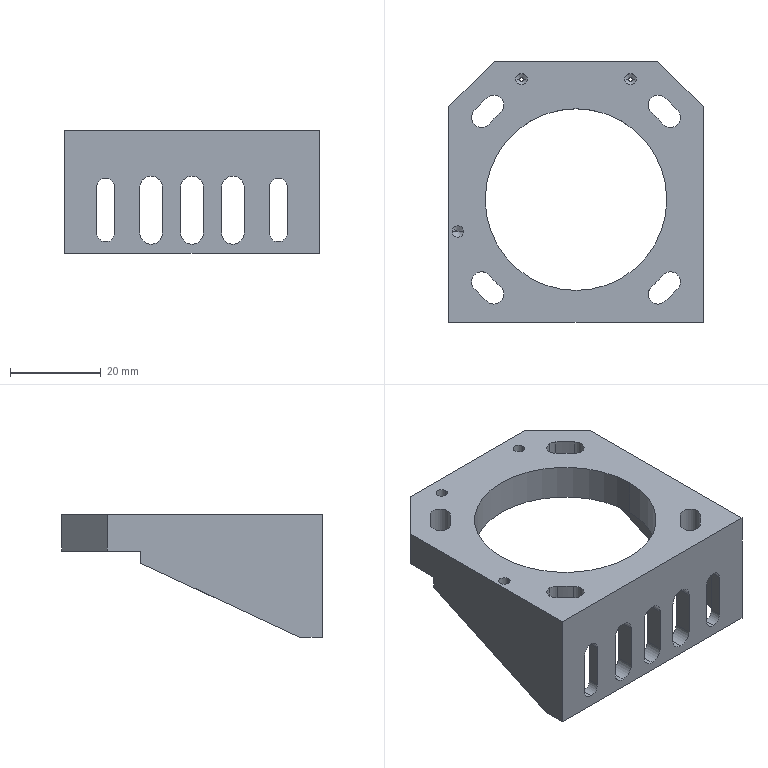NC program | NX | posted with a generic post | part box 56 x 57.4 x 27 mm
Lines 31 to 1094 of 24340:
(ZLEVEL_PROFILE , TOOL : D10C)
N54 T10 M6
N56 G54
N58 G17 G0 G90 X-33.8 Y5.489 B0. C0. S2500 M3
N60 G43 Z30. H10
N62 Z1.5
N64 G94 G1 Y28.32 Z0.303 F1000.
N66 X-33.683 Y29.131 Z0.261
N68 X-33.438 Y29.914 Z0.218
N70 X-33.071 Y30.647 Z0.175
N72 X-32.592 Y31.312 Z0.132
N74 X-32.012 Y31.892 Z0.089
N76 X-31.347 Y32.371 Z0.046
N78 X-30.614 Y32.738 Z0.003
N80 X-29.831 Y32.983 Z-0.04
N82 X-29.02 Y33.1 Z-0.083
N84 X-28.7 Z-0.1
N86 X18.7 F2500.
N88 G2 X22.306 Y31.606 R5.1
N90 G1 X32.306 Y21.606
N92 G2 X33.8 Y18. R5.1
N94 G1 Y-18.
N96 G2 X32.306 Y-21.606 R5.1
N98 G1 X22.306 Y-31.606
N100 G2 X18.7 Y-33.1 R5.1
N102 G1 X-28.7
N104 G2 X-33.8 Y-28. R5.1
N106 G1 Y28.
N108 G2 X-28.7 Y33.1 R5.1
N110 G1 X-22.971 Z-0.2
N112 X18.7
N114 G2 X22.306 Y31.606 R5.1
N116 G1 X32.306 Y21.606
N118 G2 X33.8 Y18. R5.1
N120 G1 Y-18.
N122 G2 X32.306 Y-21.606 R5.1
N124 G1 X22.306 Y-31.606
N126 G2 X18.7 Y-33.1 R5.1
N128 G1 X-28.7
N130 G2 X-33.8 Y-28. R5.1
N132 G1 Y28.
N134 G2 X-28.7 Y33.1 R5.1
N136 G1 X-22.971 Z-0.3
N138 X18.7
N140 G2 X22.306 Y31.606 R5.1
N142 G1 X32.306 Y21.606
N144 G2 X33.8 Y18. R5.1
N146 G1 Y-18.
N148 G2 X32.306 Y-21.606 R5.1
N150 G1 X22.306 Y-31.606
N152 G2 X18.7 Y-33.1 R5.1
N154 G1 X-28.7
N156 G2 X-33.8 Y-28. R5.1
N158 G1 Y28.
N160 G2 X-28.7 Y33.1 R5.1
N162 G1 X-22.971 Z-0.4
N164 X18.7
N166 G2 X22.306 Y31.606 R5.1
N168 G1 X32.306 Y21.606
N170 G2 X33.8 Y18. R5.1
N172 G1 Y-18.
N174 G2 X32.306 Y-21.606 R5.1
N176 G1 X22.306 Y-31.606
N178 G2 X18.7 Y-33.1 R5.1
N180 G1 X-28.7
N182 G2 X-33.8 Y-28. R5.1
N184 G1 Y28.
N186 G2 X-28.7 Y33.1 R5.1
N188 G1 X-22.971 Z-0.5
N190 X18.7
N192 G2 X22.306 Y31.606 R5.1
N194 G1 X32.306 Y21.606
N196 G2 X33.8 Y18. R5.1
N198 G1 Y-18.
N200 G2 X32.306 Y-21.606 R5.1
N202 G1 X22.306 Y-31.606
N204 G2 X18.7 Y-33.1 R5.1
N206 G1 X-28.7
N208 G2 X-33.8 Y-28. R5.1
N210 G1 Y28.
N212 G2 X-28.7 Y33.1 R5.1
N214 G1 X-22.971 Z-0.6
N216 X18.7
N218 G2 X22.306 Y31.606 R5.1
N220 G1 X32.306 Y21.606
N222 G2 X33.8 Y18. R5.1
N224 G1 Y-18.
N226 G2 X32.306 Y-21.606 R5.1
N228 G1 X22.306 Y-31.606
N230 G2 X18.7 Y-33.1 R5.1
N232 G1 X-28.7
N234 G2 X-33.8 Y-28. R5.1
N236 G1 Y28.
N238 G2 X-28.7 Y33.1 R5.1
N240 G1 X-22.971 Z-0.7
N242 X18.7
N244 G2 X22.306 Y31.606 R5.1
N246 G1 X32.306 Y21.606
N248 G2 X33.8 Y18. R5.1
N250 G1 Y-18.
N252 G2 X32.306 Y-21.606 R5.1
N254 G1 X22.306 Y-31.606
N256 G2 X18.7 Y-33.1 R5.1
N258 G1 X-28.7
N260 G2 X-33.8 Y-28. R5.1
N262 G1 Y28.
N264 G2 X-28.7 Y33.1 R5.1
N266 G1 X-22.971 Z-0.8
N268 X18.7
N270 G2 X22.306 Y31.606 R5.1
N272 G1 X32.306 Y21.606
N274 G2 X33.8 Y18. R5.1
N276 G1 Y-18.
N278 G2 X32.306 Y-21.606 R5.1
N280 G1 X22.306 Y-31.606
N282 G2 X18.7 Y-33.1 R5.1
N284 G1 X-28.7
N286 G2 X-33.8 Y-28. R5.1
N288 G1 Y28.
N290 G2 X-28.7 Y33.1 R5.1
N292 G1 X-22.971 Z-0.9
N294 X18.7
N296 G2 X22.306 Y31.606 R5.1
N298 G1 X32.306 Y21.606
N300 G2 X33.8 Y18. R5.1
N302 G1 Y-18.
N304 G2 X32.306 Y-21.606 R5.1
N306 G1 X22.306 Y-31.606
N308 G2 X18.7 Y-33.1 R5.1
N310 G1 X-28.7
N312 G2 X-33.8 Y-28. R5.1
N314 G1 Y28.
N316 G2 X-28.7 Y33.1 R5.1
N318 G1 X-22.971 Z-1.
N320 X18.7
N322 G2 X22.306 Y31.606 R5.1
N324 G1 X32.306 Y21.606
N326 G2 X33.8 Y18. R5.1
N328 G1 Y-18.
N330 G2 X32.306 Y-21.606 R5.1
N332 G1 X22.306 Y-31.606
N334 G2 X18.7 Y-33.1 R5.1
N336 G1 X-28.7
N338 G2 X-33.8 Y-28. R5.1
N340 G1 Y28.
N342 G2 X-28.7 Y33.1 R5.1
N344 G1 X-22.971 Z-1.1
N346 X18.7
N348 G2 X22.306 Y31.606 R5.1
N350 G1 X32.306 Y21.606
N352 G2 X33.8 Y18. R5.1
N354 G1 Y-18.
N356 G2 X32.306 Y-21.606 R5.1
N358 G1 X22.306 Y-31.606
N360 G2 X18.7 Y-33.1 R5.1
N362 G1 X-28.7
N364 G2 X-33.8 Y-28. R5.1
N366 G1 Y28.
N368 G2 X-28.7 Y33.1 R5.1
N370 G1 X-22.971 Z-1.2
N372 X18.7
N374 G2 X22.306 Y31.606 R5.1
N376 G1 X32.306 Y21.606
N378 G2 X33.8 Y18. R5.1
N380 G1 Y-18.
N382 G2 X32.306 Y-21.606 R5.1
N384 G1 X22.306 Y-31.606
N386 G2 X18.7 Y-33.1 R5.1
N388 G1 X-28.7
N390 G2 X-33.8 Y-28. R5.1
N392 G1 Y28.
N394 G2 X-28.7 Y33.1 R5.1
N396 G1 X-22.971 Z-1.3
N398 X18.7
N400 G2 X22.306 Y31.606 R5.1
N402 G1 X32.306 Y21.606
N404 G2 X33.8 Y18. R5.1
N406 G1 Y-18.
N408 G2 X32.306 Y-21.606 R5.1
N410 G1 X22.306 Y-31.606
N412 G2 X18.7 Y-33.1 R5.1
N414 G1 X-28.7
N416 G2 X-33.8 Y-28. R5.1
N418 G1 Y28.
N420 G2 X-28.7 Y33.1 R5.1
N422 G1 X-22.971 Z-1.4
N424 X18.7
N426 G2 X22.306 Y31.606 R5.1
N428 G1 X32.306 Y21.606
N430 G2 X33.8 Y18. R5.1
N432 G1 Y-18.
N434 G2 X32.306 Y-21.606 R5.1
N436 G1 X22.306 Y-31.606
N438 G2 X18.7 Y-33.1 R5.1
N440 G1 X-28.7
N442 G2 X-33.8 Y-28. R5.1
N444 G1 Y28.
N446 G2 X-28.7 Y33.1 R5.1
N448 G1 X-22.971 Z-1.5
N450 X18.7
N452 G2 X22.306 Y31.606 R5.1
N454 G1 X32.306 Y21.606
N456 G2 X33.8 Y18. R5.1
N458 G1 Y-18.
N460 G2 X32.306 Y-21.606 R5.1
N462 G1 X22.306 Y-31.606
N464 G2 X18.7 Y-33.1 R5.1
N466 G1 X-28.7
N468 G2 X-33.8 Y-28. R5.1
N470 G1 Y28.
N472 G2 X-28.7 Y33.1 R5.1
N474 G1 X-22.971 Z-1.6
N476 X18.7
N478 G2 X22.306 Y31.606 R5.1
N480 G1 X32.306 Y21.606
N482 G2 X33.8 Y18. R5.1
N484 G1 Y-18.
N486 G2 X32.306 Y-21.606 R5.1
N488 G1 X22.306 Y-31.606
N490 G2 X18.7 Y-33.1 R5.1
N492 G1 X-28.7
N494 G2 X-33.8 Y-28. R5.1
N496 G1 Y28.
N498 G2 X-28.7 Y33.1 R5.1
N500 G1 X-22.971 Z-1.7
N502 X18.7
N504 G2 X22.306 Y31.606 R5.1
N506 G1 X32.306 Y21.606
N508 G2 X33.8 Y18. R5.1
N510 G1 Y-18.
N512 G2 X32.306 Y-21.606 R5.1
N514 G1 X22.306 Y-31.606
N516 G2 X18.7 Y-33.1 R5.1
N518 G1 X-28.7
N520 G2 X-33.8 Y-28. R5.1
N522 G1 Y28.
N524 G2 X-28.7 Y33.1 R5.1
N526 G1 X-22.971 Z-1.8
N528 X18.7
N530 G2 X22.306 Y31.606 R5.1
N532 G1 X32.306 Y21.606
N534 G2 X33.8 Y18. R5.1
N536 G1 Y-18.
N538 G2 X32.306 Y-21.606 R5.1
N540 G1 X22.306 Y-31.606
N542 G2 X18.7 Y-33.1 R5.1
N544 G1 X-28.7
N546 G2 X-33.8 Y-28. R5.1
N548 G1 Y28.
N550 G2 X-28.7 Y33.1 R5.1
N552 G1 X-22.971 Z-1.9
N554 X18.7
N556 G2 X22.306 Y31.606 R5.1
N558 G1 X32.306 Y21.606
N560 G2 X33.8 Y18. R5.1
N562 G1 Y-18.
N564 G2 X32.306 Y-21.606 R5.1
N566 G1 X22.306 Y-31.606
N568 G2 X18.7 Y-33.1 R5.1
N570 G1 X-28.7
N572 G2 X-33.8 Y-28. R5.1
N574 G1 Y28.
N576 G2 X-28.7 Y33.1 R5.1
N578 G1 X-22.971 Z-2.
N580 X18.7
N582 G2 X22.306 Y31.606 R5.1
N584 G1 X32.306 Y21.606
N586 G2 X33.8 Y18. R5.1
N588 G1 Y-18.
N590 G2 X32.306 Y-21.606 R5.1
N592 G1 X22.306 Y-31.606
N594 G2 X18.7 Y-33.1 R5.1
N596 G1 X-28.7
N598 G2 X-33.8 Y-28. R5.1
N600 G1 Y28.
N602 G2 X-28.7 Y33.1 R5.1
N604 G1 X-22.971 Z-2.1
N606 X18.7
N608 G2 X22.306 Y31.606 R5.1
N610 G1 X32.306 Y21.606
N612 G2 X33.8 Y18. R5.1
N614 G1 Y-18.
N616 G2 X32.306 Y-21.606 R5.1
N618 G1 X22.306 Y-31.606
N620 G2 X18.7 Y-33.1 R5.1
N622 G1 X-28.7
N624 G2 X-33.8 Y-28. R5.1
N626 G1 Y28.
N628 G2 X-28.7 Y33.1 R5.1
N630 G1 X-22.971 Z-2.2
N632 X18.7
N634 G2 X22.306 Y31.606 R5.1
N636 G1 X32.306 Y21.606
N638 G2 X33.8 Y18. R5.1
N640 G1 Y-18.
N642 G2 X32.306 Y-21.606 R5.1
N644 G1 X22.306 Y-31.606
N646 G2 X18.7 Y-33.1 R5.1
N648 G1 X-28.7
N650 G2 X-33.8 Y-28. R5.1
N652 G1 Y28.
N654 G2 X-28.7 Y33.1 R5.1
N656 G1 X-22.971 Z-2.3
N658 X18.7
N660 G2 X22.306 Y31.606 R5.1
N662 G1 X32.306 Y21.606
N664 G2 X33.8 Y18. R5.1
N666 G1 Y-18.
N668 G2 X32.306 Y-21.606 R5.1
N670 G1 X22.306 Y-31.606
N672 G2 X18.7 Y-33.1 R5.1
N674 G1 X-28.7
N676 G2 X-33.8 Y-28. R5.1
N678 G1 Y28.
N680 G2 X-28.7 Y33.1 R5.1
N682 G1 X-22.971 Z-2.4
N684 X18.7
N686 G2 X22.306 Y31.606 R5.1
N688 G1 X32.306 Y21.606
N690 G2 X33.8 Y18. R5.1
N692 G1 Y-18.
N694 G2 X32.306 Y-21.606 R5.1
N696 G1 X22.306 Y-31.606
N698 G2 X18.7 Y-33.1 R5.1
N700 G1 X-28.7
N702 G2 X-33.8 Y-28. R5.1
N704 G1 Y28.
N706 G2 X-28.7 Y33.1 R5.1
N708 G1 X-22.971 Z-2.5
N710 X18.7
N712 G2 X22.306 Y31.606 R5.1
N714 G1 X32.306 Y21.606
N716 G2 X33.8 Y18. R5.1
N718 G1 Y-18.
N720 G2 X32.306 Y-21.606 R5.1
N722 G1 X22.306 Y-31.606
N724 G2 X18.7 Y-33.1 R5.1
N726 G1 X-28.7
N728 G2 X-33.8 Y-28. R5.1
N730 G1 Y28.
N732 G2 X-28.7 Y33.1 R5.1
N734 G1 X-22.971 Z-2.6
N736 X18.7
N738 G2 X22.306 Y31.606 R5.1
N740 G1 X32.306 Y21.606
N742 G2 X33.8 Y18. R5.1
N744 G1 Y-18.
N746 G2 X32.306 Y-21.606 R5.1
N748 G1 X22.306 Y-31.606
N750 G2 X18.7 Y-33.1 R5.1
N752 G1 X-28.7
N754 G2 X-33.8 Y-28. R5.1
N756 G1 Y28.
N758 G2 X-28.7 Y33.1 R5.1
N760 G1 X-22.971 Z-2.7
N762 X18.7
N764 G2 X22.306 Y31.606 R5.1
N766 G1 X32.306 Y21.606
N768 G2 X33.8 Y18. R5.1
N770 G1 Y-18.
N772 G2 X32.306 Y-21.606 R5.1
N774 G1 X22.306 Y-31.606
N776 G2 X18.7 Y-33.1 R5.1
N778 G1 X-28.7
N780 G2 X-33.8 Y-28. R5.1
N782 G1 Y28.
N784 G2 X-28.7 Y33.1 R5.1
N786 G1 X-22.971 Z-2.8
N788 X18.7
N790 G2 X22.306 Y31.606 R5.1
N792 G1 X32.306 Y21.606
N794 G2 X33.8 Y18. R5.1
N796 G1 Y-18.
N798 G2 X32.306 Y-21.606 R5.1
N800 G1 X22.306 Y-31.606
N802 G2 X18.7 Y-33.1 R5.1
N804 G1 X-28.7
N806 G2 X-33.8 Y-28. R5.1
N808 G1 Y28.
N810 G2 X-28.7 Y33.1 R5.1
N812 G1 X-22.971 Z-2.9
N814 X18.7
N816 G2 X22.306 Y31.606 R5.1
N818 G1 X32.306 Y21.606
N820 G2 X33.8 Y18. R5.1
N822 G1 Y-18.
N824 G2 X32.306 Y-21.606 R5.1
N826 G1 X22.306 Y-31.606
N828 G2 X18.7 Y-33.1 R5.1
N830 G1 X-28.7
N832 G2 X-33.8 Y-28. R5.1
N834 G1 Y28.
N836 G2 X-28.7 Y33.1 R5.1
N838 G1 X-22.971 Z-3.
N840 X18.7
N842 G2 X22.306 Y31.606 R5.1
N844 G1 X32.306 Y21.606
N846 G2 X33.8 Y18. R5.1
N848 G1 Y-18.
N850 G2 X32.306 Y-21.606 R5.1
N852 G1 X22.306 Y-31.606
N854 G2 X18.7 Y-33.1 R5.1
N856 G1 X-28.7
N858 G2 X-33.8 Y-28. R5.1
N860 G1 Y28.
N862 G2 X-28.7 Y33.1 R5.1
N864 G1 X-22.971 Z-3.1
N866 X18.7
N868 G2 X22.306 Y31.606 R5.1
N870 G1 X32.306 Y21.606
N872 G2 X33.8 Y18. R5.1
N874 G1 Y-18.
N876 G2 X32.306 Y-21.606 R5.1
N878 G1 X22.306 Y-31.606
N880 G2 X18.7 Y-33.1 R5.1
N882 G1 X-28.7
N884 G2 X-33.8 Y-28. R5.1
N886 G1 Y28.
N888 G2 X-28.7 Y33.1 R5.1
N890 G1 X-22.971 Z-3.2
N892 X18.7
N894 G2 X22.306 Y31.606 R5.1
N896 G1 X32.306 Y21.606
N898 G2 X33.8 Y18. R5.1
N900 G1 Y-18.
N902 G2 X32.306 Y-21.606 R5.1
N904 G1 X22.306 Y-31.606
N906 G2 X18.7 Y-33.1 R5.1
N908 G1 X-28.7
N910 G2 X-33.8 Y-28. R5.1
N912 G1 Y28.
N914 G2 X-28.7 Y33.1 R5.1
N916 G1 X-22.971 Z-3.3
N918 X18.7
N920 G2 X22.306 Y31.606 R5.1
N922 G1 X32.306 Y21.606
N924 G2 X33.8 Y18. R5.1
N926 G1 Y-18.
N928 G2 X32.306 Y-21.606 R5.1
N930 G1 X22.306 Y-31.606
N932 G2 X18.7 Y-33.1 R5.1
N934 G1 X-28.7
N936 G2 X-33.8 Y-28. R5.1
N938 G1 Y28.
N940 G2 X-28.7 Y33.1 R5.1
N942 G1 X-22.971 Z-3.4
N944 X18.7
N946 G2 X22.306 Y31.606 R5.1
N948 G1 X32.306 Y21.606
N950 G2 X33.8 Y18. R5.1
N952 G1 Y-18.
N954 G2 X32.306 Y-21.606 R5.1
N956 G1 X22.306 Y-31.606
N958 G2 X18.7 Y-33.1 R5.1
N960 G1 X-28.7
N962 G2 X-33.8 Y-28. R5.1
N964 G1 Y28.
N966 G2 X-28.7 Y33.1 R5.1
N968 G1 X-22.971 Z-3.5
N970 X18.7
N972 G2 X22.306 Y31.606 R5.1
N974 G1 X32.306 Y21.606
N976 G2 X33.8 Y18. R5.1
N978 G1 Y-18.
N980 G2 X32.306 Y-21.606 R5.1
N982 G1 X22.306 Y-31.606
N984 G2 X18.7 Y-33.1 R5.1
N986 G1 X-28.7
N988 G2 X-33.8 Y-28. R5.1
N990 G1 Y28.
N992 G2 X-28.7 Y33.1 R5.1
N994 G1 X-22.971 Z-3.6
N996 X18.7
N998 G2 X22.306 Y31.606 R5.1
N1000 G1 X32.306 Y21.606
N1002 G2 X33.8 Y18. R5.1
N1004 G1 Y-18.
N1006 G2 X32.306 Y-21.606 R5.1
N1008 G1 X22.306 Y-31.606
N1010 G2 X18.7 Y-33.1 R5.1
N1012 G1 X-28.7
N1014 G2 X-33.8 Y-28. R5.1
N1016 G1 Y28.
N1018 G2 X-28.7 Y33.1 R5.1
N1020 G1 X-22.971 Z-3.7
N1022 X18.7
N1024 G2 X22.306 Y31.606 R5.1
N1026 G1 X32.306 Y21.606
N1028 G2 X33.8 Y18. R5.1
N1030 G1 Y-18.
N1032 G2 X32.306 Y-21.606 R5.1
N1034 G1 X22.306 Y-31.606
N1036 G2 X18.7 Y-33.1 R5.1
N1038 G1 X-28.7
N1040 G2 X-33.8 Y-28. R5.1
N1042 G1 Y28.
N1044 G2 X-28.7 Y33.1 R5.1
N1046 G1 X-22.971 Z-3.8
N1048 X18.7
N1050 G2 X22.306 Y31.606 R5.1
N1052 G1 X32.306 Y21.606
N1054 G2 X33.8 Y18. R5.1
N1056 G1 Y-18.
N1058 G2 X32.306 Y-21.606 R5.1
N1060 G1 X22.306 Y-31.606
N1062 G2 X18.7 Y-33.1 R5.1
N1064 G1 X-28.7
N1066 G2 X-33.8 Y-28. R5.1
N1068 G1 Y28.
N1070 G2 X-28.7 Y33.1 R5.1
N1072 G1 X-22.971 Z-3.9
N1074 X18.7
N1076 G2 X22.306 Y31.606 R5.1
N1078 G1 X32.306 Y21.606
N1080 G2 X33.8 Y18. R5.1
N1082 G1 Y-18.
N1084 G2 X32.306 Y-21.606 R5.1
N1086 G1 X22.306 Y-31.606
N1088 G2 X18.7 Y-33.1 R5.1
N1090 G1 X-28.7
N1092 G2 X-33.8 Y-28. R5.1
N1094 G1 Y28.
N1096 G2 X-28.7 Y33.1 R5.1
N1098 G1 X-22.971 Z-4.
N1100 X18.7
N1102 G2 X22.306 Y31.606 R5.1
N1104 G1 X32.306 Y21.606
N1106 G2 X33.8 Y18. R5.1
N1108 G1 Y-18.
N1110 G2 X32.306 Y-21.606 R5.1
N1112 G1 X22.306 Y-31.606
N1114 G2 X18.7 Y-33.1 R5.1
N1116 G1 X-28.7
N1118 G2 X-33.8 Y-28. R5.1
N1120 G1 Y28.
N1122 G2 X-28.7 Y33.1 R5.1
N1124 G1 X-22.971 Z-4.1
N1126 X18.7
N1128 G2 X22.306 Y31.606 R5.1
N1130 G1 X32.306 Y21.606
N1132 G2 X33.8 Y18. R5.1
N1134 G1 Y-18.
N1136 G2 X32.306 Y-21.606 R5.1
N1138 G1 X22.306 Y-31.606
N1140 G2 X18.7 Y-33.1 R5.1
N1142 G1 X-28.7
N1144 G2 X-33.8 Y-28. R5.1
N1146 G1 Y28.
N1148 G2 X-28.7 Y33.1 R5.1
N1150 G1 X-22.971 Z-4.2
N1152 X18.7
N1154 G2 X22.306 Y31.606 R5.1
N1156 G1 X32.306 Y21.606
N1158 G2 X33.8 Y18. R5.1
N1160 G1 Y-18.
N1162 G2 X32.306 Y-21.606 R5.1
N1164 G1 X22.306 Y-31.606
N1166 G2 X18.7 Y-33.1 R5.1
N1168 G1 X-28.7
N1170 G2 X-33.8 Y-28. R5.1
N1172 G1 Y28.
N1174 G2 X-28.7 Y33.1 R5.1
N1176 G1 X-22.971 Z-4.3
N1178 X18.7
N1180 G2 X22.306 Y31.606 R5.1
N1182 G1 X32.306 Y21.606
N1184 G2 X33.8 Y18. R5.1
N1186 G1 Y-18.
N1188 G2 X32.306 Y-21.606 R5.1
N1190 G1 X22.306 Y-31.606
N1192 G2 X18.7 Y-33.1 R5.1
N1194 G1 X-28.7
N1196 G2 X-33.8 Y-28. R5.1
N1198 G1 Y28.
N1200 G2 X-28.7 Y33.1 R5.1
N1202 G1 X-22.971 Z-4.4
N1204 X18.7
N1206 G2 X22.306 Y31.606 R5.1
N1208 G1 X32.306 Y21.606
N1210 G2 X33.8 Y18. R5.1
N1212 G1 Y-18.
N1214 G2 X32.306 Y-21.606 R5.1
N1216 G1 X22.306 Y-31.606
N1218 G2 X18.7 Y-33.1 R5.1
N1220 G1 X-28.7
N1222 G2 X-33.8 Y-28. R5.1
N1224 G1 Y28.
N1226 G2 X-28.7 Y33.1 R5.1
N1228 G1 X-22.971 Z-4.5
N1230 X18.7
N1232 G2 X22.306 Y31.606 R5.1
N1234 G1 X32.306 Y21.606
N1236 G2 X33.8 Y18. R5.1
N1238 G1 Y-18.
N1240 G2 X32.306 Y-21.606 R5.1
N1242 G1 X22.306 Y-31.606
N1244 G2 X18.7 Y-33.1 R5.1
N1246 G1 X-28.7
N1248 G2 X-33.8 Y-28. R5.1
N1250 G1 Y28.
N1252 G2 X-28.7 Y33.1 R5.1
N1254 G1 X-22.971 Z-4.6
N1256 X18.7
N1258 G2 X22.306 Y31.606 R5.1
N1260 G1 X32.306 Y21.606
N1262 G2 X33.8 Y18. R5.1
N1264 G1 Y-18.
N1266 G2 X32.306 Y-21.606 R5.1
N1268 G1 X22.306 Y-31.606
N1270 G2 X18.7 Y-33.1 R5.1
N1272 G1 X-28.7
N1274 G2 X-33.8 Y-28. R5.1
N1276 G1 Y28.
N1278 G2 X-28.7 Y33.1 R5.1
N1280 G1 X-22.971 Z-4.7
N1282 X18.7
N1284 G2 X22.306 Y31.606 R5.1
N1286 G1 X32.306 Y21.606
N1288 G2 X33.8 Y18. R5.1
N1290 G1 Y-18.
N1292 G2 X32.306 Y-21.606 R5.1
N1294 G1 X22.306 Y-31.606
N1296 G2 X18.7 Y-33.1 R5.1
N1298 G1 X-28.7
N1300 G2 X-33.8 Y-28. R5.1
N1302 G1 Y28.
N1304 G2 X-28.7 Y33.1 R5.1
N1306 G1 X-22.971 Z-4.8
N1308 X18.7
N1310 G2 X22.306 Y31.606 R5.1
N1312 G1 X32.306 Y21.606
N1314 G2 X33.8 Y18. R5.1
N1316 G1 Y-18.
N1318 G2 X32.306 Y-21.606 R5.1
N1320 G1 X22.306 Y-31.606
N1322 G2 X18.7 Y-33.1 R5.1
N1324 G1 X-28.7
N1326 G2 X-33.8 Y-28. R5.1
N1328 G1 Y28.
N1330 G2 X-28.7 Y33.1 R5.1
N1332 G1 X-22.971 Z-4.9
N1334 X18.7
N1336 G2 X22.306 Y31.606 R5.1
N1338 G1 X32.306 Y21.606
N1340 G2 X33.8 Y18. R5.1
N1342 G1 Y-18.
N1344 G2 X32.306 Y-21.606 R5.1
N1346 G1 X22.306 Y-31.606
N1348 G2 X18.7 Y-33.1 R5.1
N1350 G1 X-28.7
N1352 G2 X-33.8 Y-28. R5.1
N1354 G1 Y28.
N1356 G2 X-28.7 Y33.1 R5.1
N1358 G1 X-22.971 Z-5.
N1360 X18.7
N1362 G2 X22.306 Y31.606 R5.1
N1364 G1 X32.306 Y21.606
N1366 G2 X33.8 Y18. R5.1
N1368 G1 Y-18.
N1370 G2 X32.306 Y-21.606 R5.1
N1372 G1 X22.306 Y-31.606
N1374 G2 X18.7 Y-33.1 R5.1
N1376 G1 X-28.7
N1378 G2 X-33.8 Y-28. R5.1
N1380 G1 Y28.
N1382 G2 X-28.7 Y33.1 R5.1
N1384 G1 X-22.971 Z-5.1
N1386 X18.7
N1388 G2 X22.306 Y31.606 R5.1
N1390 G1 X32.306 Y21.606
N1392 G2 X33.8 Y18. R5.1
N1394 G1 Y-18.
N1396 G2 X32.306 Y-21.606 R5.1
N1398 G1 X22.306 Y-31.606
N1400 G2 X18.7 Y-33.1 R5.1
N1402 G1 X-28.7
N1404 G2 X-33.8 Y-28. R5.1
N1406 G1 Y28.
N1408 G2 X-28.7 Y33.1 R5.1
N1410 G1 X-22.971 Z-5.2
N1412 X18.7
N1414 G2 X22.306 Y31.606 R5.1
N1416 G1 X32.306 Y21.606
N1418 G2 X33.8 Y18. R5.1
N1420 G1 Y-18.
N1422 G2 X32.306 Y-21.606 R5.1
N1424 G1 X22.306 Y-31.606
N1426 G2 X18.7 Y-33.1 R5.1
N1428 G1 X-28.7
N1430 G2 X-33.8 Y-28. R5.1
N1432 G1 Y28.
N1434 G2 X-28.7 Y33.1 R5.1
N1436 G1 X-22.971 Z-5.3
N1438 X18.7
N1440 G2 X22.306 Y31.606 R5.1
N1442 G1 X32.306 Y21.606
N1444 G2 X33.8 Y18. R5.1
N1446 G1 Y-18.
N1448 G2 X32.306 Y-21.606 R5.1
N1450 G1 X22.306 Y-31.606
N1452 G2 X18.7 Y-33.1 R5.1
N1454 G1 X-28.7
N1456 G2 X-33.8 Y-28. R5.1
N1458 G1 Y28.
N1460 G2 X-28.7 Y33.1 R5.1
N1462 G1 X-22.971 Z-5.4
N1464 X18.7
N1466 G2 X22.306 Y31.606 R5.1
N1468 G1 X32.306 Y21.606
N1470 G2 X33.8 Y18. R5.1
N1472 G1 Y-18.
N1474 G2 X32.306 Y-21.606 R5.1
N1476 G1 X22.306 Y-31.606
N1478 G2 X18.7 Y-33.1 R5.1
N1480 G1 X-28.7
N1482 G2 X-33.8 Y-28. R5.1
N1484 G1 Y28.
N1486 G2 X-28.7 Y33.1 R5.1
N1488 G1 X-22.971 Z-5.5
N1490 X18.7
N1492 G2 X22.306 Y31.606 R5.1
N1494 G1 X32.306 Y21.606
N1496 G2 X33.8 Y18. R5.1
N1498 G1 Y-18.
N1500 G2 X32.306 Y-21.606 R5.1
N1502 G1 X22.306 Y-31.606
N1504 G2 X18.7 Y-33.1 R5.1
N1506 G1 X-28.7
N1508 G2 X-33.8 Y-28. R5.1
N1510 G1 Y28.
N1512 G2 X-28.7 Y33.1 R5.1
N1514 G1 X-22.971 Z-5.6
N1516 X18.7
N1518 G2 X22.306 Y31.606 R5.1
N1520 G1 X32.306 Y21.606
N1522 G2 X33.8 Y18. R5.1
N1524 G1 Y-18.
N1526 G2 X32.306 Y-21.606 R5.1
N1528 G1 X22.306 Y-31.606
N1530 G2 X18.7 Y-33.1 R5.1
N1532 G1 X-28.7
N1534 G2 X-33.8 Y-28. R5.1
N1536 G1 Y28.
N1538 G2 X-28.7 Y33.1 R5.1
N1540 G1 X-22.971 Z-5.7
N1542 X18.7
N1544 G2 X22.306 Y31.606 R5.1
N1546 G1 X32.306 Y21.606
N1548 G2 X33.8 Y18. R5.1
N1550 G1 Y-18.
N1552 G2 X32.306 Y-21.606 R5.1
N1554 G1 X22.306 Y-31.606
N1556 G2 X18.7 Y-33.1 R5.1
N1558 G1 X-28.7
N1560 G2 X-33.8 Y-28. R5.1
N1562 G1 Y28.
N1564 G2 X-28.7 Y33.1 R5.1
N1566 G1 X-22.971 Z-5.8
N1568 X18.7
N1570 G2 X22.306 Y31.606 R5.1
N1572 G1 X32.306 Y21.606
N1574 G2 X33.8 Y18. R5.1
N1576 G1 Y-18.
N1578 G2 X32.306 Y-21.606 R5.1
N1580 G1 X22.306 Y-31.606
N1582 G2 X18.7 Y-33.1 R5.1
N1584 G1 X-28.7
N1586 G2 X-33.8 Y-28. R5.1
N1588 G1 Y28.
N1590 G2 X-28.7 Y33.1 R5.1
N1592 G1 X-22.971 Z-5.9
N1594 X18.7
N1596 G2 X22.306 Y31.606 R5.1
N1598 G1 X32.306 Y21.606
N1600 G2 X33.8 Y18. R5.1
N1602 G1 Y-18.
N1604 G2 X32.306 Y-21.606 R5.1
N1606 G1 X22.306 Y-31.606
N1608 G2 X18.7 Y-33.1 R5.1
N1610 G1 X-28.7
N1612 G2 X-33.8 Y-28. R5.1
N1614 G1 Y28.
N1616 G2 X-28.7 Y33.1 R5.1
N1618 G1 X-22.971 Z-6.
N1620 X18.7
N1622 G2 X22.306 Y31.606 R5.1
N1624 G1 X32.306 Y21.606
N1626 G2 X33.8 Y18. R5.1
N1628 G1 Y-18.
N1630 G2 X32.306 Y-21.606 R5.1
N1632 G1 X22.306 Y-31.606
N1634 G2 X18.7 Y-33.1 R5.1
N1636 G1 X-28.7
N1638 G2 X-33.8 Y-28. R5.1
N1640 G1 Y28.
N1642 G2 X-28.7 Y33.1 R5.1
N1644 G1 X-22.971 Z-6.1
N1646 X18.7
N1648 G2 X22.306 Y31.606 R5.1
N1650 G1 X32.306 Y21.606
N1652 G2 X33.8 Y18. R5.1
N1654 G1 Y-18.
N1656 G2 X32.306 Y-21.606 R5.1
N1658 G1 X22.306 Y-31.606
N1660 G2 X18.7 Y-33.1 R5.1
N1662 G1 X-28.7
N1664 G2 X-33.8 Y-28. R5.1
N1666 G1 Y28.
N1668 G2 X-28.7 Y33.1 R5.1
N1670 G1 X-22.971 Z-6.2
N1672 X18.7
N1674 G2 X22.306 Y31.606 R5.1
N1676 G1 X32.306 Y21.606
N1678 G2 X33.8 Y18. R5.1
N1680 G1 Y-18.
N1682 G2 X32.306 Y-21.606 R5.1
N1684 G1 X22.306 Y-31.606
N1686 G2 X18.7 Y-33.1 R5.1
N1688 G1 X-28.7
N1690 G2 X-33.8 Y-28. R5.1
N1692 G1 Y28.
N1694 G2 X-28.7 Y33.1 R5.1
N1696 G1 X-22.971 Z-6.3
N1698 X18.7
N1700 G2 X22.306 Y31.606 R5.1
N1702 G1 X32.306 Y21.606
N1704 G2 X33.8 Y18. R5.1
N1706 G1 Y-18.
N1708 G2 X32.306 Y-21.606 R5.1
N1710 G1 X22.306 Y-31.606
N1712 G2 X18.7 Y-33.1 R5.1
N1714 G1 X-28.7
N1716 G2 X-33.8 Y-28. R5.1
N1718 G1 Y28.
N1720 G2 X-28.7 Y33.1 R5.1
N1722 G1 X-22.971 Z-6.4
N1724 X18.7
N1726 G2 X22.306 Y31.606 R5.1
N1728 G1 X32.306 Y21.606
N1730 G2 X33.8 Y18. R5.1
N1732 G1 Y-18.
N1734 G2 X32.306 Y-21.606 R5.1
N1736 G1 X22.306 Y-31.606
N1738 G2 X18.7 Y-33.1 R5.1
N1740 G1 X-28.7
N1742 G2 X-33.8 Y-28. R5.1
N1744 G1 Y28.
N1746 G2 X-28.7 Y33.1 R5.1
N1748 G1 X-22.971 Z-6.5
N1750 X18.7
N1752 G2 X22.306 Y31.606 R5.1
N1754 G1 X32.306 Y21.606
N1756 G2 X33.8 Y18. R5.1
N1758 G1 Y-18.
N1760 G2 X32.306 Y-21.606 R5.1
N1762 G1 X22.306 Y-31.606
N1764 G2 X18.7 Y-33.1 R5.1
N1766 G1 X-28.7
N1768 G2 X-33.8 Y-28. R5.1
N1770 G1 Y28.
N1772 G2 X-28.7 Y33.1 R5.1
N1774 G1 X-22.971 Z-6.6
N1776 X18.7
N1778 G2 X22.306 Y31.606 R5.1
N1780 G1 X32.306 Y21.606
N1782 G2 X33.8 Y18. R5.1
N1784 G1 Y-18.
N1786 G2 X32.306 Y-21.606 R5.1
N1788 G1 X22.306 Y-31.606
N1790 G2 X18.7 Y-33.1 R5.1
N1792 G1 X-28.7
N1794 G2 X-33.8 Y-28. R5.1
N1796 G1 Y28.
N1798 G2 X-28.7 Y33.1 R5.1
N1800 G1 X-22.971 Z-6.7
N1802 X18.7
N1804 G2 X22.306 Y31.606 R5.1
N1806 G1 X32.306 Y21.606
N1808 G2 X33.8 Y18. R5.1
N1810 G1 Y-18.
N1812 G2 X32.306 Y-21.606 R5.1
N1814 G1 X22.306 Y-31.606
N1816 G2 X18.7 Y-33.1 R5.1
N1818 G1 X-28.7
N1820 G2 X-33.8 Y-28. R5.1
N1822 G1 Y28.
N1824 G2 X-28.7 Y33.1 R5.1
N1826 G1 X-22.971 Z-6.8
N1828 X18.7
N1830 G2 X22.306 Y31.606 R5.1
N1832 G1 X32.306 Y21.606
N1834 G2 X33.8 Y18. R5.1
N1836 G1 Y-18.
N1838 G2 X32.306 Y-21.606 R5.1
N1840 G1 X22.306 Y-31.606
N1842 G2 X18.7 Y-33.1 R5.1
N1844 G1 X-28.7
N1846 G2 X-33.8 Y-28. R5.1
N1848 G1 Y28.
N1850 G2 X-28.7 Y33.1 R5.1
N1852 G1 X-22.971 Z-6.9
N1854 X18.7
N1856 G2 X22.306 Y31.606 R5.1
N1858 G1 X32.306 Y21.606
N1860 G2 X33.8 Y18. R5.1
N1862 G1 Y-18.
N1864 G2 X32.306 Y-21.606 R5.1
N1866 G1 X22.306 Y-31.606
N1868 G2 X18.7 Y-33.1 R5.1
N1870 G1 X-28.7
N1872 G2 X-33.8 Y-28. R5.1
N1874 G1 Y28.
N1876 G2 X-28.7 Y33.1 R5.1
N1878 G1 X-22.971 Z-7.
N1880 X18.7
N1882 G2 X22.306 Y31.606 R5.1
N1884 G1 X32.306 Y21.606
N1886 G2 X33.8 Y18. R5.1
N1888 G1 Y-18.
N1890 G2 X32.306 Y-21.606 R5.1
N1892 G1 X22.306 Y-31.606
N1894 G2 X18.7 Y-33.1 R5.1
N1896 G1 X-28.7
N1898 G2 X-33.8 Y-28. R5.1
N1900 G1 Y28.
N1902 G2 X-28.7 Y33.1 R5.1
N1904 G1 X-22.971 Z-7.1
N1906 X18.7
N1908 G2 X22.306 Y31.606 R5.1
N1910 G1 X32.306 Y21.606
N1912 G2 X33.8 Y18. R5.1
N1914 G1 Y-18.
N1916 G2 X32.306 Y-21.606 R5.1
N1918 G1 X22.306 Y-31.606
N1920 G2 X18.7 Y-33.1 R5.1
N1922 G1 X-28.7
N1924 G2 X-33.8 Y-28. R5.1
N1926 G1 Y28.
N1928 G2 X-28.7 Y33.1 R5.1
N1930 G1 X-22.971 Z-7.2
N1932 X18.7
N1934 G2 X22.306 Y31.606 R5.1
N1936 G1 X32.306 Y21.606
N1938 G2 X33.8 Y18. R5.1
N1940 G1 Y-18.
N1942 G2 X32.306 Y-21.606 R5.1
N1944 G1 X22.306 Y-31.606
N1946 G2 X18.7 Y-33.1 R5.1
N1948 G1 X-28.7
N1950 G2 X-33.8 Y-28. R5.1
N1952 G1 Y28.
N1954 G2 X-28.7 Y33.1 R5.1
N1956 G1 X-22.971 Z-7.3
N1958 X18.7
N1960 G2 X22.306 Y31.606 R5.1
N1962 G1 X32.306 Y21.606
N1964 G2 X33.8 Y18. R5.1
N1966 G1 Y-18.
N1968 G2 X32.306 Y-21.606 R5.1
N1970 G1 X22.306 Y-31.606
N1972 G2 X18.7 Y-33.1 R5.1
N1974 G1 X-28.7
N1976 G2 X-33.8 Y-28. R5.1
N1978 G1 Y28.
N1980 G2 X-28.7 Y33.1 R5.1
N1982 G1 X-22.971 Z-7.4
N1984 X18.7
N1986 G2 X22.306 Y31.606 R5.1
N1988 G1 X32.306 Y21.606
N1990 G2 X33.8 Y18. R5.1
N1992 G1 Y-18.
N1994 G2 X32.306 Y-21.606 R5.1
N1996 G1 X22.306 Y-31.606
N1998 G2 X18.7 Y-33.1 R5.1
N2000 G1 X-28.7
N2002 G2 X-33.8 Y-28. R5.1
N2004 G1 Y28.
N2006 G2 X-28.7 Y33.1 R5.1
N2008 G1 X-22.971 Z-7.5
N2010 X18.7
N2012 G2 X22.306 Y31.606 R5.1
N2014 G1 X32.306 Y21.606
N2016 G2 X33.8 Y18. R5.1
N2018 G1 Y-18.
N2020 G2 X32.306 Y-21.606 R5.1
N2022 G1 X22.306 Y-31.606
N2024 G2 X18.7 Y-33.1 R5.1
N2026 G1 X-28.7
N2028 G2 X-33.8 Y-28. R5.1
N2030 G1 Y28.
N2032 G2 X-28.7 Y33.1 R5.1
N2034 G1 X-22.971 Z-7.6
N2036 X18.7
N2038 G2 X22.306 Y31.606 R5.1
N2040 G1 X32.306 Y21.606
N2042 G2 X33.8 Y18. R5.1
N2044 G1 Y-18.
N2046 G2 X32.306 Y-21.606 R5.1
N2048 G1 X22.306 Y-31.606
N2050 G2 X18.7 Y-33.1 R5.1
N2052 G1 X-28.7
N2054 G2 X-33.8 Y-28. R5.1
N2056 G1 Y28.
N2058 G2 X-28.7 Y33.1 R5.1
N2060 G1 X-22.971 Z-7.7
N2062 X18.7
N2064 G2 X22.306 Y31.606 R5.1
N2066 G1 X32.306 Y21.606
N2068 G2 X33.8 Y18. R5.1
N2070 G1 Y-18.
N2072 G2 X32.306 Y-21.606 R5.1
N2074 G1 X22.306 Y-31.606
N2076 G2 X18.7 Y-33.1 R5.1
N2078 G1 X-28.7
N2080 G2 X-33.8 Y-28. R5.1
N2082 G1 Y28.
N2084 G2 X-28.7 Y33.1 R5.1
N2086 G1 X-22.971 Z-7.8
N2088 X18.7
N2090 G2 X22.306 Y31.606 R5.1
N2092 G1 X32.306 Y21.606
N2094 G2 X33.8 Y18. R5.1
N2096 G1 Y-18.
N2098 G2 X32.306 Y-21.606 R5.1
N2100 G1 X22.306 Y-31.606
N2102 G2 X18.7 Y-33.1 R5.1
N2104 G1 X-28.7
N2106 G2 X-33.8 Y-28. R5.1
N2108 G1 Y28.
N2110 G2 X-28.7 Y33.1 R5.1
N2112 G1 X-22.971 Z-7.9
N2114 X18.7
N2116 G2 X22.306 Y31.606 R5.1
N2118 G1 X32.306 Y21.606
N2120 G2 X33.8 Y18. R5.1
N2122 G1 Y-18.
N2124 G2 X32.306 Y-21.606 R5.1
N2126 G1 X22.306 Y-31.606
N2128 G2 X18.7 Y-33.1 R5.1
N2130 G1 X-28.7
N2132 G2 X-33.8 Y-28. R5.1
N2134 G1 Y28.
N2136 G2 X-28.7 Y33.1 R5.1
N2138 G1 X-22.971 Z-8.
N2140 X18.7
N2142 G2 X22.306 Y31.606 R5.1
N2144 G1 X32.306 Y21.606
N2146 G2 X33.8 Y18. R5.1
N2148 G1 Y-18.
N2150 G2 X32.306 Y-21.606 R5.1
N2152 G1 X22.306 Y-31.606
N2154 G2 X18.7 Y-33.1 R5.1
N2156 G1 X-28.7
N2158 G2 X-33.8 Y-28. R5.1
N2160 G1 Y28.
N2162 G2 X-28.7 Y33.1 R5.1
N2164 G1 X-22.971 Z-8.1
N2166 X18.7
N2168 G2 X22.306 Y31.606 R5.1
N2170 G1 X32.306 Y21.606
N2172 G2 X33.8 Y18. R5.1
N2174 G1 Y-18.